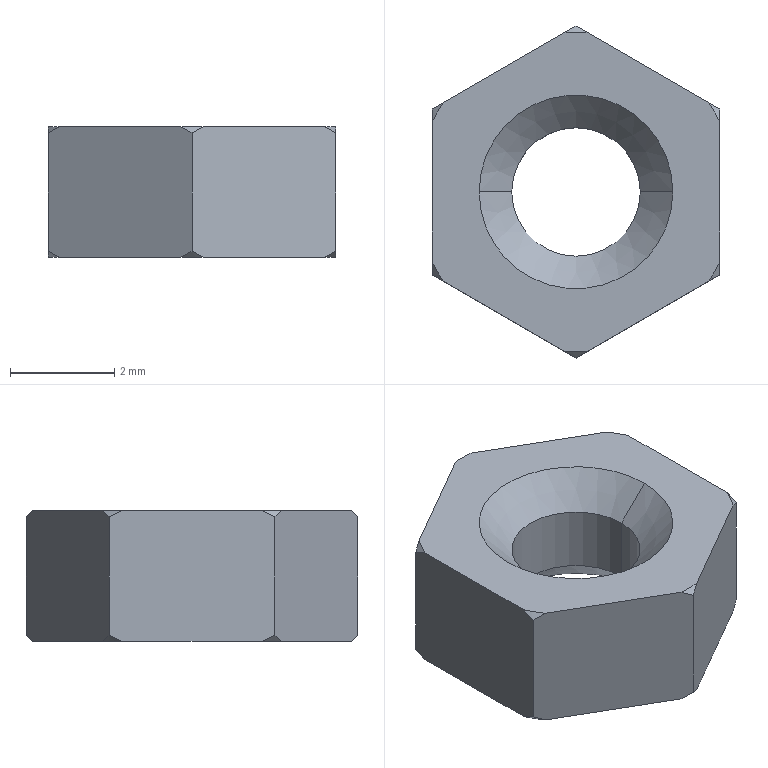Part | NX | features BREP 1 | 1 solid | 26 faces | box 5.5 x 6.351 x 2.5 mm | volume 50.092 mm3 | cone 16 | plane 8 | cylinder 2 | commonest cylinder face diameters 2.459 x2
STEP:
#1=CARTESIAN_POINT('',(-1.23,0.,-1.876));
#2=VERTEX_POINT('',#1);
#3=CARTESIAN_POINT('',(1.23,0.,-1.876));
#4=VERTEX_POINT('',#3);
#5=CARTESIAN_POINT('',(0.,0.,-1.876));
#6=DIRECTION('',(0.,0.,1.));
#7=DIRECTION('',(1.,0.,0.));
#8=AXIS2_PLACEMENT_3D('',#5,#6,#7);
#9=CIRCLE('',#8,1.23);
#10=EDGE_CURVE('',#2,#4,#9,.T.);
#11=ORIENTED_EDGE('',*,*,#10,.T.);
#12=CARTESIAN_POINT('',(1.854,0.,-2.5));
#13=VERTEX_POINT('',#12);
#14=CARTESIAN_POINT('',(1.23,0.,-1.876));
#15=DIRECTION('',(0.7071,0.,-0.7071));
#16=VECTOR('',#15,1000.);
#17=LINE('',#14,#16);
#18=EDGE_CURVE('',#13,#4,#17,.F.);
#19=ORIENTED_EDGE('',*,*,#18,.F.);
#20=CARTESIAN_POINT('',(-1.854,0.,-2.5));
#21=VERTEX_POINT('',#20);
#22=CARTESIAN_POINT('',(0.,0.,-2.5));
#23=DIRECTION('',(0.,0.,1.));
#24=DIRECTION('',(1.,0.,0.));
#25=AXIS2_PLACEMENT_3D('',#22,#23,#24);
#26=CIRCLE('',#25,1.854);
#27=EDGE_CURVE('',#21,#13,#26,.T.);
#28=ORIENTED_EDGE('',*,*,#27,.F.);
#29=CARTESIAN_POINT('',(-1.23,0.,-1.876));
#30=DIRECTION('',(-0.7071,0.,-0.7071));
#31=VECTOR('',#30,1000.);
#32=LINE('',#29,#31);
#33=EDGE_CURVE('',#21,#2,#32,.F.);
#34=ORIENTED_EDGE('',*,*,#33,.T.);
#35=EDGE_LOOP('',(#11,#19,#28,#34));
#36=FACE_BOUND('',#35,.T.);
#37=CARTESIAN_POINT('',(0.,0.,-1.876));
#38=DIRECTION('',(0.,0.,-1.));
#39=DIRECTION('',(1.,0.,0.));
#40=AXIS2_PLACEMENT_3D('',#37,#38,#39);
#41=CONICAL_SURFACE('',#40,1.23,0.7854);
#42=ADVANCED_FACE('',(#36),#41,.F.);
#43=ORIENTED_EDGE('',*,*,#10,.F.);
#44=CARTESIAN_POINT('',(-1.23,0.,-0.6241));
#45=VERTEX_POINT('',#44);
#46=CARTESIAN_POINT('',(-1.23,0.,-17.));
#47=DIRECTION('',(0.,0.,1.));
#48=VECTOR('',#47,1000.);
#49=LINE('',#46,#48);
#50=EDGE_CURVE('',#2,#45,#49,.T.);
#51=ORIENTED_EDGE('',*,*,#50,.T.);
#52=CARTESIAN_POINT('',(1.23,0.,-0.6241));
#53=VERTEX_POINT('',#52);
#54=CARTESIAN_POINT('',(0.,0.,-0.6241));
#55=DIRECTION('',(0.,0.,1.));
#56=DIRECTION('',(1.,0.,0.));
#57=AXIS2_PLACEMENT_3D('',#54,#55,#56);
#58=CIRCLE('',#57,1.23);
#59=EDGE_CURVE('',#45,#53,#58,.T.);
#60=ORIENTED_EDGE('',*,*,#59,.T.);
#61=CARTESIAN_POINT('',(1.23,0.,-17.));
#62=DIRECTION('',(0.,0.,1.));
#63=VECTOR('',#62,1000.);
#64=LINE('',#61,#63);
#65=EDGE_CURVE('',#4,#53,#64,.T.);
#66=ORIENTED_EDGE('',*,*,#65,.F.);
#67=EDGE_LOOP('',(#43,#51,#60,#66));
#68=FACE_BOUND('',#67,.T.);
#69=CARTESIAN_POINT('',(0.,0.,-17.));
#70=DIRECTION('',(0.,0.,1.));
#71=DIRECTION('',(-1.,0.,0.));
#72=AXIS2_PLACEMENT_3D('',#69,#70,#71);
#73=CYLINDRICAL_SURFACE('',#72,1.23);
#74=ADVANCED_FACE('',(#68),#73,.F.);
#75=ORIENTED_EDGE('',*,*,#59,.F.);
#76=CARTESIAN_POINT('',(-1.854,0.,0.));
#77=VERTEX_POINT('',#76);
#78=CARTESIAN_POINT('',(-1.854,0.,0.));
#79=DIRECTION('',(-0.7071,0.,0.7071));
#80=VECTOR('',#79,1000.);
#81=LINE('',#78,#80);
#82=EDGE_CURVE('',#45,#77,#81,.T.);
#83=ORIENTED_EDGE('',*,*,#82,.T.);
#84=CARTESIAN_POINT('',(1.854,0.,0.));
#85=VERTEX_POINT('',#84);
#86=CARTESIAN_POINT('',(0.,0.,0.));
#87=DIRECTION('',(0.,0.,1.));
#88=DIRECTION('',(1.,0.,0.));
#89=AXIS2_PLACEMENT_3D('',#86,#87,#88);
#90=CIRCLE('',#89,1.854);
#91=EDGE_CURVE('',#77,#85,#90,.T.);
#92=ORIENTED_EDGE('',*,*,#91,.T.);
#93=CARTESIAN_POINT('',(1.854,0.,0.));
#94=DIRECTION('',(0.7071,0.,0.7071));
#95=VECTOR('',#94,1000.);
#96=LINE('',#93,#95);
#97=EDGE_CURVE('',#53,#85,#96,.T.);
#98=ORIENTED_EDGE('',*,*,#97,.F.);
#99=EDGE_LOOP('',(#75,#83,#92,#98));
#100=FACE_BOUND('',#99,.T.);
#101=CARTESIAN_POINT('',(0.,0.,0.));
#102=DIRECTION('',(0.,0.,1.));
#103=DIRECTION('',(-1.,0.,0.));
#104=AXIS2_PLACEMENT_3D('',#101,#102,#103);
#105=CONICAL_SURFACE('',#104,1.854,0.7854);
#106=ADVANCED_FACE('',(#100),#105,.F.);
#107=CARTESIAN_POINT('',(-2.75,1.344,0.));
#108=VERTEX_POINT('',#107);
#109=CARTESIAN_POINT('',(-2.75,1.588,-0.1147));
#110=VERTEX_POINT('',#109);
#111=CARTESIAN_POINT('',(-2.75,1.344,0.));
#112=CARTESIAN_POINT('',(-2.75,1.426,-0.03612));
#113=CARTESIAN_POINT('',(-2.75,1.507,-0.07447));
#114=CARTESIAN_POINT('',(-2.75,1.588,-0.1147));
#115=B_SPLINE_CURVE_WITH_KNOTS('',3,(#111,#112,#113,#114),.UNSPECIFIED.,.F.,.F.,(4,4),(0.,1.),.PIECEWISE_BEZIER_KNOTS.);
#116=EDGE_CURVE('',#108,#110,#115,.T.);
#117=ORIENTED_EDGE('',*,*,#116,.F.);
#118=CARTESIAN_POINT('',(-2.539,1.71,0.));
#119=VERTEX_POINT('',#118);
#120=CARTESIAN_POINT('',(0.,0.,0.));
#121=DIRECTION('',(0.,0.,1.));
#122=DIRECTION('',(1.,0.,0.));
#123=AXIS2_PLACEMENT_3D('',#120,#121,#122);
#124=CIRCLE('',#123,3.061);
#125=EDGE_CURVE('',#119,#108,#124,.T.);
#126=ORIENTED_EDGE('',*,*,#125,.F.);
#127=CARTESIAN_POINT('',(-2.75,1.588,-0.1147));
#128=CARTESIAN_POINT('',(-2.68,1.628,-0.07445));
#129=CARTESIAN_POINT('',(-2.61,1.669,-0.03611));
#130=CARTESIAN_POINT('',(-2.539,1.71,0.));
#131=B_SPLINE_CURVE_WITH_KNOTS('',3,(#127,#128,#129,#130),.UNSPECIFIED.,.F.,.F.,(4,4),(0.,1.),.PIECEWISE_BEZIER_KNOTS.);
#132=EDGE_CURVE('',#110,#119,#131,.T.);
#133=ORIENTED_EDGE('',*,*,#132,.F.);
#134=EDGE_LOOP('',(#117,#126,#133));
#135=FACE_BOUND('',#134,.T.);
#136=CARTESIAN_POINT('',(0.,0.,-0.5893));
#137=DIRECTION('',(0.,0.,-1.));
#138=DIRECTION('',(1.,0.,0.));
#139=AXIS2_PLACEMENT_3D('',#136,#137,#138);
#140=CONICAL_SURFACE('',#139,3.65,0.7854);
#141=ADVANCED_FACE('',(#135),#140,.T.);
#142=CARTESIAN_POINT('',(-0.2113,3.053,0.));
#143=VERTEX_POINT('',#142);
#144=CARTESIAN_POINT('',(0.,3.175,-0.1147));
#145=VERTEX_POINT('',#144);
#146=CARTESIAN_POINT('',(-0.2113,3.053,0.));
#147=CARTESIAN_POINT('',(-0.1398,3.095,-0.03624));
#148=CARTESIAN_POINT('',(-0.06943,3.135,-0.07459));
#149=CARTESIAN_POINT('',(0.,3.175,-0.1147));
#150=B_SPLINE_CURVE_WITH_KNOTS('',3,(#146,#147,#148,#149),.UNSPECIFIED.,.F.,.F.,(4,4),(0.,1.),.PIECEWISE_BEZIER_KNOTS.);
#151=EDGE_CURVE('',#143,#145,#150,.T.);
#152=ORIENTED_EDGE('',*,*,#151,.F.);
#153=CARTESIAN_POINT('',(0.2113,3.053,0.));
#154=VERTEX_POINT('',#153);
#155=CARTESIAN_POINT('',(0.,0.,0.));
#156=DIRECTION('',(0.,0.,1.));
#157=DIRECTION('',(1.,0.,0.));
#158=AXIS2_PLACEMENT_3D('',#155,#156,#157);
#159=CIRCLE('',#158,3.061);
#160=EDGE_CURVE('',#154,#143,#159,.T.);
#161=ORIENTED_EDGE('',*,*,#160,.F.);
#162=CARTESIAN_POINT('',(0.,3.175,-0.1147));
#163=CARTESIAN_POINT('',(0.06968,3.135,-0.07445));
#164=CARTESIAN_POINT('',(0.1401,3.095,-0.03611));
#165=CARTESIAN_POINT('',(0.2113,3.053,0.));
#166=B_SPLINE_CURVE_WITH_KNOTS('',3,(#162,#163,#164,#165),.UNSPECIFIED.,.F.,.F.,(4,4),(0.,1.),.PIECEWISE_BEZIER_KNOTS.);
#167=EDGE_CURVE('',#145,#154,#166,.T.);
#168=ORIENTED_EDGE('',*,*,#167,.F.);
#169=EDGE_LOOP('',(#152,#161,#168));
#170=FACE_BOUND('',#169,.T.);
#171=CARTESIAN_POINT('',(0.,0.,-0.5893));
#172=DIRECTION('',(0.,0.,-1.));
#173=DIRECTION('',(1.,0.,0.));
#174=AXIS2_PLACEMENT_3D('',#171,#172,#173);
#175=CONICAL_SURFACE('',#174,3.65,0.7854);
#176=ADVANCED_FACE('',(#170),#175,.T.);
#177=CARTESIAN_POINT('',(2.539,1.71,0.));
#178=VERTEX_POINT('',#177);
#179=CARTESIAN_POINT('',(2.75,1.588,-0.1147));
#180=VERTEX_POINT('',#179);
#181=CARTESIAN_POINT('',(2.539,1.71,0.));
#182=CARTESIAN_POINT('',(2.61,1.668,-0.03624));
#183=CARTESIAN_POINT('',(2.681,1.628,-0.07459));
#184=CARTESIAN_POINT('',(2.75,1.588,-0.1147));
#185=B_SPLINE_CURVE_WITH_KNOTS('',3,(#181,#182,#183,#184),.UNSPECIFIED.,.F.,.F.,(4,4),(0.,1.),.PIECEWISE_BEZIER_KNOTS.);
#186=EDGE_CURVE('',#178,#180,#185,.T.);
#187=ORIENTED_EDGE('',*,*,#186,.F.);
#188=CARTESIAN_POINT('',(2.75,1.344,0.));
#189=VERTEX_POINT('',#188);
#190=CARTESIAN_POINT('',(0.,0.,0.));
#191=DIRECTION('',(0.,0.,1.));
#192=DIRECTION('',(1.,0.,0.));
#193=AXIS2_PLACEMENT_3D('',#190,#191,#192);
#194=CIRCLE('',#193,3.061);
#195=EDGE_CURVE('',#189,#178,#194,.T.);
#196=ORIENTED_EDGE('',*,*,#195,.F.);
#197=CARTESIAN_POINT('',(2.75,1.588,-0.1147));
#198=CARTESIAN_POINT('',(2.75,1.507,-0.07455));
#199=CARTESIAN_POINT('',(2.75,1.426,-0.03607));
#200=CARTESIAN_POINT('',(2.75,1.344,0.));
#201=B_SPLINE_CURVE_WITH_KNOTS('',3,(#197,#198,#199,#200),.UNSPECIFIED.,.F.,.F.,(4,4),(0.,1.),.PIECEWISE_BEZIER_KNOTS.);
#202=EDGE_CURVE('',#180,#189,#201,.T.);
#203=ORIENTED_EDGE('',*,*,#202,.F.);
#204=EDGE_LOOP('',(#187,#196,#203));
#205=FACE_BOUND('',#204,.T.);
#206=CARTESIAN_POINT('',(0.,0.,-0.5893));
#207=DIRECTION('',(0.,0.,-1.));
#208=DIRECTION('',(1.,0.,0.));
#209=AXIS2_PLACEMENT_3D('',#206,#207,#208);
#210=CONICAL_SURFACE('',#209,3.65,0.7854);
#211=ADVANCED_FACE('',(#205),#210,.T.);
#212=CARTESIAN_POINT('',(2.75,-1.344,0.));
#213=VERTEX_POINT('',#212);
#214=CARTESIAN_POINT('',(2.75,-1.588,-0.1147));
#215=VERTEX_POINT('',#214);
#216=CARTESIAN_POINT('',(2.75,-1.344,0.));
#217=CARTESIAN_POINT('',(2.75,-1.426,-0.03612));
#218=CARTESIAN_POINT('',(2.75,-1.507,-0.07447));
#219=CARTESIAN_POINT('',(2.75,-1.588,-0.1147));
#220=B_SPLINE_CURVE_WITH_KNOTS('',3,(#216,#217,#218,#219),.UNSPECIFIED.,.F.,.F.,(4,4),(0.,1.),.PIECEWISE_BEZIER_KNOTS.);
#221=EDGE_CURVE('',#213,#215,#220,.T.);
#222=ORIENTED_EDGE('',*,*,#221,.F.);
#223=CARTESIAN_POINT('',(2.539,-1.71,0.));
#224=VERTEX_POINT('',#223);
#225=CARTESIAN_POINT('',(0.,0.,0.));
#226=DIRECTION('',(0.,0.,1.));
#227=DIRECTION('',(1.,0.,0.));
#228=AXIS2_PLACEMENT_3D('',#225,#226,#227);
#229=CIRCLE('',#228,3.061);
#230=EDGE_CURVE('',#224,#213,#229,.T.);
#231=ORIENTED_EDGE('',*,*,#230,.F.);
#232=CARTESIAN_POINT('',(2.75,-1.588,-0.1147));
#233=CARTESIAN_POINT('',(2.68,-1.628,-0.07445));
#234=CARTESIAN_POINT('',(2.61,-1.669,-0.03611));
#235=CARTESIAN_POINT('',(2.539,-1.71,0.));
#236=B_SPLINE_CURVE_WITH_KNOTS('',3,(#232,#233,#234,#235),.UNSPECIFIED.,.F.,.F.,(4,4),(0.,1.),.PIECEWISE_BEZIER_KNOTS.);
#237=EDGE_CURVE('',#215,#224,#236,.T.);
#238=ORIENTED_EDGE('',*,*,#237,.F.);
#239=EDGE_LOOP('',(#222,#231,#238));
#240=FACE_BOUND('',#239,.T.);
#241=CARTESIAN_POINT('',(0.,0.,-0.5893));
#242=DIRECTION('',(0.,0.,-1.));
#243=DIRECTION('',(1.,0.,0.));
#244=AXIS2_PLACEMENT_3D('',#241,#242,#243);
#245=CONICAL_SURFACE('',#244,3.65,0.7854);
#246=ADVANCED_FACE('',(#240),#245,.T.);
#247=CARTESIAN_POINT('',(0.2113,-3.053,0.));
#248=VERTEX_POINT('',#247);
#249=CARTESIAN_POINT('',(0.,-3.175,-0.1147));
#250=VERTEX_POINT('',#249);
#251=CARTESIAN_POINT('',(0.2113,-3.053,0.));
#252=CARTESIAN_POINT('',(0.1398,-3.095,-0.03624));
#253=CARTESIAN_POINT('',(0.06943,-3.135,-0.07459));
#254=CARTESIAN_POINT('',(0.,-3.175,-0.1147));
#255=B_SPLINE_CURVE_WITH_KNOTS('',3,(#251,#252,#253,#254),.UNSPECIFIED.,.F.,.F.,(4,4),(0.,1.),.PIECEWISE_BEZIER_KNOTS.);
#256=EDGE_CURVE('',#248,#250,#255,.T.);
#257=ORIENTED_EDGE('',*,*,#256,.F.);
#258=CARTESIAN_POINT('',(-0.2113,-3.053,0.));
#259=VERTEX_POINT('',#258);
#260=CARTESIAN_POINT('',(0.,0.,0.));
#261=DIRECTION('',(0.,0.,1.));
#262=DIRECTION('',(1.,0.,0.));
#263=AXIS2_PLACEMENT_3D('',#260,#261,#262);
#264=CIRCLE('',#263,3.061);
#265=EDGE_CURVE('',#259,#248,#264,.T.);
#266=ORIENTED_EDGE('',*,*,#265,.F.);
#267=CARTESIAN_POINT('',(0.,-3.175,-0.1147));
#268=CARTESIAN_POINT('',(-0.06968,-3.135,-0.07445));
#269=CARTESIAN_POINT('',(-0.1401,-3.095,-0.03611));
#270=CARTESIAN_POINT('',(-0.2113,-3.053,0.));
#271=B_SPLINE_CURVE_WITH_KNOTS('',3,(#267,#268,#269,#270),.UNSPECIFIED.,.F.,.F.,(4,4),(0.,1.),.PIECEWISE_BEZIER_KNOTS.);
#272=EDGE_CURVE('',#250,#259,#271,.T.);
#273=ORIENTED_EDGE('',*,*,#272,.F.);
#274=EDGE_LOOP('',(#257,#266,#273));
#275=FACE_BOUND('',#274,.T.);
#276=CARTESIAN_POINT('',(0.,0.,-0.5893));
#277=DIRECTION('',(0.,0.,-1.));
#278=DIRECTION('',(1.,0.,0.));
#279=AXIS2_PLACEMENT_3D('',#276,#277,#278);
#280=CONICAL_SURFACE('',#279,3.65,0.7854);
#281=ADVANCED_FACE('',(#275),#280,.T.);
#282=CARTESIAN_POINT('',(-2.75,-1.588,-0.1147));
#283=VERTEX_POINT('',#282);
#284=CARTESIAN_POINT('',(-2.75,-1.344,0.));
#285=VERTEX_POINT('',#284);
#286=CARTESIAN_POINT('',(-2.75,-1.588,-0.1147));
#287=CARTESIAN_POINT('',(-2.75,-1.507,-0.07455));
#288=CARTESIAN_POINT('',(-2.75,-1.426,-0.03607));
#289=CARTESIAN_POINT('',(-2.75,-1.344,0.));
#290=B_SPLINE_CURVE_WITH_KNOTS('',3,(#286,#287,#288,#289),.UNSPECIFIED.,.F.,.F.,(4,4),(0.,1.),.PIECEWISE_BEZIER_KNOTS.);
#291=EDGE_CURVE('',#283,#285,#290,.T.);
#292=ORIENTED_EDGE('',*,*,#291,.F.);
#293=CARTESIAN_POINT('',(-2.539,-1.71,0.));
#294=VERTEX_POINT('',#293);
#295=CARTESIAN_POINT('',(-2.539,-1.71,0.));
#296=CARTESIAN_POINT('',(-2.61,-1.668,-0.03624));
#297=CARTESIAN_POINT('',(-2.681,-1.628,-0.07459));
#298=CARTESIAN_POINT('',(-2.75,-1.588,-0.1147));
#299=B_SPLINE_CURVE_WITH_KNOTS('',3,(#295,#296,#297,#298),.UNSPECIFIED.,.F.,.F.,(4,4),(0.,1.),.PIECEWISE_BEZIER_KNOTS.);
#300=EDGE_CURVE('',#294,#283,#299,.T.);
#301=ORIENTED_EDGE('',*,*,#300,.F.);
#302=CARTESIAN_POINT('',(0.,0.,0.));
#303=DIRECTION('',(0.,0.,1.));
#304=DIRECTION('',(1.,0.,0.));
#305=AXIS2_PLACEMENT_3D('',#302,#303,#304);
#306=CIRCLE('',#305,3.061);
#307=EDGE_CURVE('',#285,#294,#306,.T.);
#308=ORIENTED_EDGE('',*,*,#307,.F.);
#309=EDGE_LOOP('',(#292,#301,#308));
#310=FACE_BOUND('',#309,.T.);
#311=CARTESIAN_POINT('',(0.,0.,-0.5893));
#312=DIRECTION('',(0.,0.,-1.));
#313=DIRECTION('',(1.,0.,0.));
#314=AXIS2_PLACEMENT_3D('',#311,#312,#313);
#315=CONICAL_SURFACE('',#314,3.65,0.7854);
#316=ADVANCED_FACE('',(#310),#315,.T.);
#317=CARTESIAN_POINT('',(0.,0.,0.));
#318=DIRECTION('',(0.,0.,1.));
#319=DIRECTION('',(1.,0.,0.));
#320=AXIS2_PLACEMENT_3D('',#317,#318,#319);
#321=CIRCLE('',#320,1.854);
#322=EDGE_CURVE('',#85,#77,#321,.T.);
#323=ORIENTED_EDGE('',*,*,#322,.F.);
#324=ORIENTED_EDGE('',*,*,#91,.F.);
#325=EDGE_LOOP('',(#323,#324));
#326=FACE_BOUND('',#325,.T.);
#327=CARTESIAN_POINT('',(-2.75,1.588,0.));
#328=DIRECTION('',(0.,-1.,0.));
#329=VECTOR('',#328,1000.);
#330=LINE('',#327,#329);
#331=EDGE_CURVE('',#108,#285,#330,.T.);
#332=ORIENTED_EDGE('',*,*,#331,.T.);
#333=ORIENTED_EDGE('',*,*,#307,.T.);
#334=CARTESIAN_POINT('',(-2.75,-1.588,0.));
#335=DIRECTION('',(0.866,-0.5,0.));
#336=VECTOR('',#335,1000.);
#337=LINE('',#334,#336);
#338=EDGE_CURVE('',#294,#259,#337,.T.);
#339=ORIENTED_EDGE('',*,*,#338,.T.);
#340=ORIENTED_EDGE('',*,*,#265,.T.);
#341=CARTESIAN_POINT('',(0.,-3.175,0.));
#342=DIRECTION('',(0.866,0.5,0.));
#343=VECTOR('',#342,1000.);
#344=LINE('',#341,#343);
#345=EDGE_CURVE('',#248,#224,#344,.T.);
#346=ORIENTED_EDGE('',*,*,#345,.T.);
#347=ORIENTED_EDGE('',*,*,#230,.T.);
#348=CARTESIAN_POINT('',(2.75,-1.588,0.));
#349=DIRECTION('',(0.,1.,0.));
#350=VECTOR('',#349,1000.);
#351=LINE('',#348,#350);
#352=EDGE_CURVE('',#213,#189,#351,.T.);
#353=ORIENTED_EDGE('',*,*,#352,.T.);
#354=ORIENTED_EDGE('',*,*,#195,.T.);
#355=CARTESIAN_POINT('',(2.75,1.588,0.));
#356=DIRECTION('',(-0.866,0.5,0.));
#357=VECTOR('',#356,1000.);
#358=LINE('',#355,#357);
#359=EDGE_CURVE('',#178,#154,#358,.T.);
#360=ORIENTED_EDGE('',*,*,#359,.T.);
#361=ORIENTED_EDGE('',*,*,#160,.T.);
#362=CARTESIAN_POINT('',(0.,3.175,0.));
#363=DIRECTION('',(-0.866,-0.5,0.));
#364=VECTOR('',#363,1000.);
#365=LINE('',#362,#364);
#366=EDGE_CURVE('',#143,#119,#365,.T.);
#367=ORIENTED_EDGE('',*,*,#366,.T.);
#368=ORIENTED_EDGE('',*,*,#125,.T.);
#369=EDGE_LOOP('',(#332,#333,#339,#340,#346,#347,#353,#354,#360,#361,#367,#368));
#370=FACE_BOUND('',#369,.T.);
#371=CARTESIAN_POINT('',(0.,3.061,0.));
#372=DIRECTION('',(0.,0.,-1.));
#373=DIRECTION('',(1.,0.,0.));
#374=AXIS2_PLACEMENT_3D('',#371,#372,#373);
#375=PLANE('',#374);
#376=ADVANCED_FACE('',(#326,#370),#375,.F.);
#377=ORIENTED_EDGE('',*,*,#27,.T.);
#378=CARTESIAN_POINT('',(0.,0.,-2.5));
#379=DIRECTION('',(0.,0.,1.));
#380=DIRECTION('',(1.,0.,0.));
#381=AXIS2_PLACEMENT_3D('',#378,#379,#380);
#382=CIRCLE('',#381,1.854);
#383=EDGE_CURVE('',#13,#21,#382,.T.);
#384=ORIENTED_EDGE('',*,*,#383,.T.);
#385=EDGE_LOOP('',(#377,#384));
#386=FACE_BOUND('',#385,.T.);
#387=CARTESIAN_POINT('',(-2.75,1.344,-2.5));
#388=VERTEX_POINT('',#387);
#389=CARTESIAN_POINT('',(-2.75,-1.344,-2.5));
#390=VERTEX_POINT('',#389);
#391=CARTESIAN_POINT('',(-2.75,1.854,-2.5));
#392=DIRECTION('',(0.,-1.,0.));
#393=VECTOR('',#392,1000.);
#394=LINE('',#391,#393);
#395=EDGE_CURVE('',#388,#390,#394,.T.);
#396=ORIENTED_EDGE('',*,*,#395,.F.);
#397=CARTESIAN_POINT('',(-2.539,1.71,-2.5));
#398=VERTEX_POINT('',#397);
#399=CARTESIAN_POINT('',(0.,0.,-2.5));
#400=DIRECTION('',(0.,0.,1.));
#401=DIRECTION('',(1.,0.,0.));
#402=AXIS2_PLACEMENT_3D('',#399,#400,#401);
#403=CIRCLE('',#402,3.061);
#404=EDGE_CURVE('',#398,#388,#403,.T.);
#405=ORIENTED_EDGE('',*,*,#404,.F.);
#406=CARTESIAN_POINT('',(-0.2113,3.053,-2.5));
#407=VERTEX_POINT('',#406);
#408=CARTESIAN_POINT('',(-0.5724,2.845,-2.5));
#409=DIRECTION('',(-0.866,-0.5,0.));
#410=VECTOR('',#409,1000.);
#411=LINE('',#408,#410);
#412=EDGE_CURVE('',#407,#398,#411,.T.);
#413=ORIENTED_EDGE('',*,*,#412,.F.);
#414=CARTESIAN_POINT('',(0.2113,3.053,-2.5));
#415=VERTEX_POINT('',#414);
#416=CARTESIAN_POINT('',(0.,0.,-2.5));
#417=DIRECTION('',(0.,0.,1.));
#418=DIRECTION('',(1.,0.,0.));
#419=AXIS2_PLACEMENT_3D('',#416,#417,#418);
#420=CIRCLE('',#419,3.061);
#421=EDGE_CURVE('',#415,#407,#420,.T.);
#422=ORIENTED_EDGE('',*,*,#421,.F.);
#423=CARTESIAN_POINT('',(2.539,1.71,-2.5));
#424=VERTEX_POINT('',#423);
#425=CARTESIAN_POINT('',(0.5724,2.845,-2.5));
#426=DIRECTION('',(-0.866,0.5,0.));
#427=VECTOR('',#426,1000.);
#428=LINE('',#425,#427);
#429=EDGE_CURVE('',#424,#415,#428,.T.);
#430=ORIENTED_EDGE('',*,*,#429,.F.);
#431=CARTESIAN_POINT('',(2.75,1.344,-2.5));
#432=VERTEX_POINT('',#431);
#433=CARTESIAN_POINT('',(0.,0.,-2.5));
#434=DIRECTION('',(0.,0.,1.));
#435=DIRECTION('',(1.,0.,0.));
#436=AXIS2_PLACEMENT_3D('',#433,#434,#435);
#437=CIRCLE('',#436,3.061);
#438=EDGE_CURVE('',#432,#424,#437,.T.);
#439=ORIENTED_EDGE('',*,*,#438,.F.);
#440=CARTESIAN_POINT('',(2.75,-1.344,-2.5));
#441=VERTEX_POINT('',#440);
#442=CARTESIAN_POINT('',(2.75,1.854,-2.5));
#443=DIRECTION('',(0.,1.,0.));
#444=VECTOR('',#443,1000.);
#445=LINE('',#442,#444);
#446=EDGE_CURVE('',#441,#432,#445,.T.);
#447=ORIENTED_EDGE('',*,*,#446,.F.);
#448=CARTESIAN_POINT('',(2.539,-1.71,-2.5));
#449=VERTEX_POINT('',#448);
#450=CARTESIAN_POINT('',(0.,0.,-2.5));
#451=DIRECTION('',(0.,0.,1.));
#452=DIRECTION('',(1.,0.,0.));
#453=AXIS2_PLACEMENT_3D('',#450,#451,#452);
#454=CIRCLE('',#453,3.061);
#455=EDGE_CURVE('',#449,#441,#454,.T.);
#456=ORIENTED_EDGE('',*,*,#455,.F.);
#457=CARTESIAN_POINT('',(0.2113,-3.053,-2.5));
#458=VERTEX_POINT('',#457);
#459=CARTESIAN_POINT('',(2.178,-1.918,-2.5));
#460=DIRECTION('',(0.866,0.5,0.));
#461=VECTOR('',#460,1000.);
#462=LINE('',#459,#461);
#463=EDGE_CURVE('',#458,#449,#462,.T.);
#464=ORIENTED_EDGE('',*,*,#463,.F.);
#465=CARTESIAN_POINT('',(-0.2113,-3.053,-2.5));
#466=VERTEX_POINT('',#465);
#467=CARTESIAN_POINT('',(0.,0.,-2.5));
#468=DIRECTION('',(0.,0.,1.));
#469=DIRECTION('',(1.,0.,0.));
#470=AXIS2_PLACEMENT_3D('',#467,#468,#469);
#471=CIRCLE('',#470,3.061);
#472=EDGE_CURVE('',#466,#458,#471,.T.);
#473=ORIENTED_EDGE('',*,*,#472,.F.);
#474=CARTESIAN_POINT('',(-2.539,-1.71,-2.5));
#475=VERTEX_POINT('',#474);
#476=CARTESIAN_POINT('',(-2.178,-1.918,-2.5));
#477=DIRECTION('',(0.866,-0.5,0.));
#478=VECTOR('',#477,1000.);
#479=LINE('',#476,#478);
#480=EDGE_CURVE('',#475,#466,#479,.T.);
#481=ORIENTED_EDGE('',*,*,#480,.F.);
#482=CARTESIAN_POINT('',(0.,0.,-2.5));
#483=DIRECTION('',(0.,0.,1.));
#484=DIRECTION('',(1.,0.,0.));
#485=AXIS2_PLACEMENT_3D('',#482,#483,#484);
#486=CIRCLE('',#485,3.061);
#487=EDGE_CURVE('',#390,#475,#486,.T.);
#488=ORIENTED_EDGE('',*,*,#487,.F.);
#489=EDGE_LOOP('',(#396,#405,#413,#422,#430,#439,#447,#456,#464,#473,#481,#488));
#490=FACE_BOUND('',#489,.T.);
#491=CARTESIAN_POINT('',(0.,1.854,-2.5));
#492=DIRECTION('',(0.,0.,1.));
#493=DIRECTION('',(-1.,0.,0.));
#494=AXIS2_PLACEMENT_3D('',#491,#492,#493);
#495=PLANE('',#494);
#496=ADVANCED_FACE('',(#386,#490),#495,.F.);
#497=CARTESIAN_POINT('',(-2.75,1.588,-2.385));
#498=VERTEX_POINT('',#497);
#499=CARTESIAN_POINT('',(-2.75,1.588,-2.385));
#500=CARTESIAN_POINT('',(-2.75,1.507,-2.425));
#501=CARTESIAN_POINT('',(-2.75,1.426,-2.464));
#502=CARTESIAN_POINT('',(-2.75,1.344,-2.5));
#503=B_SPLINE_CURVE_WITH_KNOTS('',3,(#499,#500,#501,#502),.UNSPECIFIED.,.F.,.F.,(4,4),(0.,1.),.PIECEWISE_BEZIER_KNOTS.);
#504=EDGE_CURVE('',#498,#388,#503,.T.);
#505=ORIENTED_EDGE('',*,*,#504,.F.);
#506=CARTESIAN_POINT('',(-2.539,1.71,-2.5));
#507=CARTESIAN_POINT('',(-2.61,1.668,-2.464));
#508=CARTESIAN_POINT('',(-2.681,1.628,-2.425));
#509=CARTESIAN_POINT('',(-2.75,1.588,-2.385));
#510=B_SPLINE_CURVE_WITH_KNOTS('',3,(#506,#507,#508,#509),.UNSPECIFIED.,.F.,.F.,(4,4),(0.,1.),.PIECEWISE_BEZIER_KNOTS.);
#511=EDGE_CURVE('',#398,#498,#510,.T.);
#512=ORIENTED_EDGE('',*,*,#511,.F.);
#513=ORIENTED_EDGE('',*,*,#404,.T.);
#514=EDGE_LOOP('',(#505,#512,#513));
#515=FACE_BOUND('',#514,.T.);
#516=CARTESIAN_POINT('',(0.,0.,-2.5));
#517=DIRECTION('',(0.,0.,1.));
#518=DIRECTION('',(-1.,0.,0.));
#519=AXIS2_PLACEMENT_3D('',#516,#517,#518);
#520=CONICAL_SURFACE('',#519,3.061,0.7854);
#521=ADVANCED_FACE('',(#515),#520,.T.);
#522=CARTESIAN_POINT('',(0.,3.175,-2.385));
#523=VERTEX_POINT('',#522);
#524=CARTESIAN_POINT('',(0.,3.175,-2.385));
#525=CARTESIAN_POINT('',(-0.06968,3.135,-2.426));
#526=CARTESIAN_POINT('',(-0.1401,3.095,-2.464));
#527=CARTESIAN_POINT('',(-0.2113,3.053,-2.5));
#528=B_SPLINE_CURVE_WITH_KNOTS('',3,(#524,#525,#526,#527),.UNSPECIFIED.,.F.,.F.,(4,4),(0.,1.),.PIECEWISE_BEZIER_KNOTS.);
#529=EDGE_CURVE('',#523,#407,#528,.T.);
#530=ORIENTED_EDGE('',*,*,#529,.F.);
#531=CARTESIAN_POINT('',(0.2113,3.053,-2.5));
#532=CARTESIAN_POINT('',(0.1398,3.095,-2.464));
#533=CARTESIAN_POINT('',(0.06943,3.135,-2.425));
#534=CARTESIAN_POINT('',(0.,3.175,-2.385));
#535=B_SPLINE_CURVE_WITH_KNOTS('',3,(#531,#532,#533,#534),.UNSPECIFIED.,.F.,.F.,(4,4),(0.,1.),.PIECEWISE_BEZIER_KNOTS.);
#536=EDGE_CURVE('',#415,#523,#535,.T.);
#537=ORIENTED_EDGE('',*,*,#536,.F.);
#538=ORIENTED_EDGE('',*,*,#421,.T.);
#539=EDGE_LOOP('',(#530,#537,#538));
#540=FACE_BOUND('',#539,.T.);
#541=CARTESIAN_POINT('',(0.,0.,-2.5));
#542=DIRECTION('',(0.,0.,1.));
#543=DIRECTION('',(-1.,0.,0.));
#544=AXIS2_PLACEMENT_3D('',#541,#542,#543);
#545=CONICAL_SURFACE('',#544,3.061,0.7854);
#546=ADVANCED_FACE('',(#540),#545,.T.);
#547=CARTESIAN_POINT('',(2.75,1.588,-2.385));
#548=VERTEX_POINT('',#547);
#549=CARTESIAN_POINT('',(2.75,1.588,-2.385));
#550=CARTESIAN_POINT('',(2.68,1.628,-2.426));
#551=CARTESIAN_POINT('',(2.61,1.669,-2.464));
#552=CARTESIAN_POINT('',(2.539,1.71,-2.5));
#553=B_SPLINE_CURVE_WITH_KNOTS('',3,(#549,#550,#551,#552),.UNSPECIFIED.,.F.,.F.,(4,4),(0.,1.),.PIECEWISE_BEZIER_KNOTS.);
#554=EDGE_CURVE('',#548,#424,#553,.T.);
#555=ORIENTED_EDGE('',*,*,#554,.F.);
#556=CARTESIAN_POINT('',(2.75,1.344,-2.5));
#557=CARTESIAN_POINT('',(2.75,1.426,-2.464));
#558=CARTESIAN_POINT('',(2.75,1.507,-2.426));
#559=CARTESIAN_POINT('',(2.75,1.588,-2.385));
#560=B_SPLINE_CURVE_WITH_KNOTS('',3,(#556,#557,#558,#559),.UNSPECIFIED.,.F.,.F.,(4,4),(0.,1.),.PIECEWISE_BEZIER_KNOTS.);
#561=EDGE_CURVE('',#432,#548,#560,.T.);
#562=ORIENTED_EDGE('',*,*,#561,.F.);
#563=ORIENTED_EDGE('',*,*,#438,.T.);
#564=EDGE_LOOP('',(#555,#562,#563));
#565=FACE_BOUND('',#564,.T.);
#566=CARTESIAN_POINT('',(0.,0.,-2.5));
#567=DIRECTION('',(0.,0.,1.));
#568=DIRECTION('',(-1.,0.,0.));
#569=AXIS2_PLACEMENT_3D('',#566,#567,#568);
#570=CONICAL_SURFACE('',#569,3.061,0.7854);
#571=ADVANCED_FACE('',(#565),#570,.T.);
#572=CARTESIAN_POINT('',(2.75,-1.588,-2.385));
#573=VERTEX_POINT('',#572);
#574=CARTESIAN_POINT('',(2.75,-1.588,-2.385));
#575=CARTESIAN_POINT('',(2.75,-1.507,-2.425));
#576=CARTESIAN_POINT('',(2.75,-1.426,-2.464));
#577=CARTESIAN_POINT('',(2.75,-1.344,-2.5));
#578=B_SPLINE_CURVE_WITH_KNOTS('',3,(#574,#575,#576,#577),.UNSPECIFIED.,.F.,.F.,(4,4),(0.,1.),.PIECEWISE_BEZIER_KNOTS.);
#579=EDGE_CURVE('',#573,#441,#578,.T.);
#580=ORIENTED_EDGE('',*,*,#579,.F.);
#581=CARTESIAN_POINT('',(2.539,-1.71,-2.5));
#582=CARTESIAN_POINT('',(2.61,-1.668,-2.464));
#583=CARTESIAN_POINT('',(2.681,-1.628,-2.425));
#584=CARTESIAN_POINT('',(2.75,-1.588,-2.385));
#585=B_SPLINE_CURVE_WITH_KNOTS('',3,(#581,#582,#583,#584),.UNSPECIFIED.,.F.,.F.,(4,4),(0.,1.),.PIECEWISE_BEZIER_KNOTS.);
#586=EDGE_CURVE('',#449,#573,#585,.T.);
#587=ORIENTED_EDGE('',*,*,#586,.F.);
#588=ORIENTED_EDGE('',*,*,#455,.T.);
#589=EDGE_LOOP('',(#580,#587,#588));
#590=FACE_BOUND('',#589,.T.);
#591=CARTESIAN_POINT('',(0.,0.,-2.5));
#592=DIRECTION('',(0.,0.,1.));
#593=DIRECTION('',(-1.,0.,0.));
#594=AXIS2_PLACEMENT_3D('',#591,#592,#593);
#595=CONICAL_SURFACE('',#594,3.061,0.7854);
#596=ADVANCED_FACE('',(#590),#595,.T.);
#597=CARTESIAN_POINT('',(-2.75,-1.588,-2.385));
#598=VERTEX_POINT('',#597);
#599=CARTESIAN_POINT('',(-2.75,-1.344,-2.5));
#600=CARTESIAN_POINT('',(-2.75,-1.426,-2.464));
#601=CARTESIAN_POINT('',(-2.75,-1.507,-2.426));
#602=CARTESIAN_POINT('',(-2.75,-1.588,-2.385));
#603=B_SPLINE_CURVE_WITH_KNOTS('',3,(#599,#600,#601,#602),.UNSPECIFIED.,.F.,.F.,(4,4),(0.,1.),.PIECEWISE_BEZIER_KNOTS.);
#604=EDGE_CURVE('',#390,#598,#603,.T.);
#605=ORIENTED_EDGE('',*,*,#604,.F.);
#606=ORIENTED_EDGE('',*,*,#487,.T.);
#607=CARTESIAN_POINT('',(-2.75,-1.588,-2.385));
#608=CARTESIAN_POINT('',(-2.68,-1.628,-2.426));
#609=CARTESIAN_POINT('',(-2.61,-1.669,-2.464));
#610=CARTESIAN_POINT('',(-2.539,-1.71,-2.5));
#611=B_SPLINE_CURVE_WITH_KNOTS('',3,(#607,#608,#609,#610),.UNSPECIFIED.,.F.,.F.,(4,4),(0.,1.),.PIECEWISE_BEZIER_KNOTS.);
#612=EDGE_CURVE('',#598,#475,#611,.T.);
#613=ORIENTED_EDGE('',*,*,#612,.F.);
#614=EDGE_LOOP('',(#605,#606,#613));
#615=FACE_BOUND('',#614,.T.);
#616=CARTESIAN_POINT('',(0.,0.,-2.5));
#617=DIRECTION('',(0.,0.,1.));
#618=DIRECTION('',(-1.,0.,0.));
#619=AXIS2_PLACEMENT_3D('',#616,#617,#618);
#620=CONICAL_SURFACE('',#619,3.061,0.7854);
#621=ADVANCED_FACE('',(#615),#620,.T.);
#622=CARTESIAN_POINT('',(0.,-3.175,-2.385));
#623=VERTEX_POINT('',#622);
#624=CARTESIAN_POINT('',(0.,-3.175,-2.385));
#625=CARTESIAN_POINT('',(0.06968,-3.135,-2.426));
#626=CARTESIAN_POINT('',(0.1401,-3.095,-2.464));
#627=CARTESIAN_POINT('',(0.2113,-3.053,-2.5));
#628=B_SPLINE_CURVE_WITH_KNOTS('',3,(#624,#625,#626,#627),.UNSPECIFIED.,.F.,.F.,(4,4),(0.,1.),.PIECEWISE_BEZIER_KNOTS.);
#629=EDGE_CURVE('',#623,#458,#628,.T.);
#630=ORIENTED_EDGE('',*,*,#629,.F.);
#631=CARTESIAN_POINT('',(-0.2113,-3.053,-2.5));
#632=CARTESIAN_POINT('',(-0.1398,-3.095,-2.464));
#633=CARTESIAN_POINT('',(-0.06943,-3.135,-2.425));
#634=CARTESIAN_POINT('',(0.,-3.175,-2.385));
#635=B_SPLINE_CURVE_WITH_KNOTS('',3,(#631,#632,#633,#634),.UNSPECIFIED.,.F.,.F.,(4,4),(0.,1.),.PIECEWISE_BEZIER_KNOTS.);
#636=EDGE_CURVE('',#466,#623,#635,.T.);
#637=ORIENTED_EDGE('',*,*,#636,.F.);
#638=ORIENTED_EDGE('',*,*,#472,.T.);
#639=EDGE_LOOP('',(#630,#637,#638));
#640=FACE_BOUND('',#639,.T.);
#641=CARTESIAN_POINT('',(0.,0.,-2.5));
#642=DIRECTION('',(0.,0.,1.));
#643=DIRECTION('',(-1.,0.,0.));
#644=AXIS2_PLACEMENT_3D('',#641,#642,#643);
#645=CONICAL_SURFACE('',#644,3.061,0.7854);
#646=ADVANCED_FACE('',(#640),#645,.T.);
#647=ORIENTED_EDGE('',*,*,#82,.F.);
#648=CARTESIAN_POINT('',(0.,0.,-0.6241));
#649=DIRECTION('',(0.,0.,1.));
#650=DIRECTION('',(1.,0.,0.));
#651=AXIS2_PLACEMENT_3D('',#648,#649,#650);
#652=CIRCLE('',#651,1.23);
#653=EDGE_CURVE('',#53,#45,#652,.T.);
#654=ORIENTED_EDGE('',*,*,#653,.F.);
#655=ORIENTED_EDGE('',*,*,#97,.T.);
#656=ORIENTED_EDGE('',*,*,#322,.T.);
#657=EDGE_LOOP('',(#647,#654,#655,#656));
#658=FACE_BOUND('',#657,.T.);
#659=CARTESIAN_POINT('',(0.,0.,0.));
#660=DIRECTION('',(0.,0.,1.));
#661=DIRECTION('',(-1.,0.,0.));
#662=AXIS2_PLACEMENT_3D('',#659,#660,#661);
#663=CONICAL_SURFACE('',#662,1.854,0.7854);
#664=ADVANCED_FACE('',(#658),#663,.F.);
#665=ORIENTED_EDGE('',*,*,#50,.F.);
#666=CARTESIAN_POINT('',(0.,0.,-1.876));
#667=DIRECTION('',(0.,0.,1.));
#668=DIRECTION('',(1.,0.,0.));
#669=AXIS2_PLACEMENT_3D('',#666,#667,#668);
#670=CIRCLE('',#669,1.23);
#671=EDGE_CURVE('',#4,#2,#670,.T.);
#672=ORIENTED_EDGE('',*,*,#671,.F.);
#673=ORIENTED_EDGE('',*,*,#65,.T.);
#674=ORIENTED_EDGE('',*,*,#653,.T.);
#675=EDGE_LOOP('',(#665,#672,#673,#674));
#676=FACE_BOUND('',#675,.T.);
#677=CARTESIAN_POINT('',(0.,0.,-17.));
#678=DIRECTION('',(0.,0.,1.));
#679=DIRECTION('',(-1.,0.,0.));
#680=AXIS2_PLACEMENT_3D('',#677,#678,#679);
#681=CYLINDRICAL_SURFACE('',#680,1.23);
#682=ADVANCED_FACE('',(#676),#681,.F.);
#683=ORIENTED_EDGE('',*,*,#18,.T.);
#684=ORIENTED_EDGE('',*,*,#671,.T.);
#685=ORIENTED_EDGE('',*,*,#33,.F.);
#686=ORIENTED_EDGE('',*,*,#383,.F.);
#687=EDGE_LOOP('',(#683,#684,#685,#686));
#688=FACE_BOUND('',#687,.T.);
#689=CARTESIAN_POINT('',(0.,0.,-1.876));
#690=DIRECTION('',(0.,0.,-1.));
#691=DIRECTION('',(1.,0.,0.));
#692=AXIS2_PLACEMENT_3D('',#689,#690,#691);
#693=CONICAL_SURFACE('',#692,1.23,0.7854);
#694=ADVANCED_FACE('',(#688),#693,.F.);
#695=ORIENTED_EDGE('',*,*,#291,.T.);
#696=ORIENTED_EDGE('',*,*,#331,.F.);
#697=ORIENTED_EDGE('',*,*,#116,.T.);
#698=CARTESIAN_POINT('',(-2.75,1.588,-4.));
#699=DIRECTION('',(0.,0.,1.));
#700=VECTOR('',#699,1000.);
#701=LINE('',#698,#700);
#702=EDGE_CURVE('',#498,#110,#701,.T.);
#703=ORIENTED_EDGE('',*,*,#702,.F.);
#704=ORIENTED_EDGE('',*,*,#504,.T.);
#705=ORIENTED_EDGE('',*,*,#395,.T.);
#706=ORIENTED_EDGE('',*,*,#604,.T.);
#707=CARTESIAN_POINT('',(-2.75,-1.588,-4.));
#708=DIRECTION('',(0.,0.,1.));
#709=VECTOR('',#708,1000.);
#710=LINE('',#707,#709);
#711=EDGE_CURVE('',#598,#283,#710,.T.);
#712=ORIENTED_EDGE('',*,*,#711,.T.);
#713=EDGE_LOOP('',(#695,#696,#697,#703,#704,#705,#706,#712));
#714=FACE_BOUND('',#713,.T.);
#715=CARTESIAN_POINT('',(-2.75,1.588,-4.));
#716=DIRECTION('',(-1.,0.,0.));
#717=DIRECTION('',(0.,0.,-1.));
#718=AXIS2_PLACEMENT_3D('',#715,#716,#717);
#719=PLANE('',#718);
#720=ADVANCED_FACE('',(#714),#719,.T.);
#721=ORIENTED_EDGE('',*,*,#132,.T.);
#722=ORIENTED_EDGE('',*,*,#366,.F.);
#723=ORIENTED_EDGE('',*,*,#151,.T.);
#724=CARTESIAN_POINT('',(0.,3.175,-4.));
#725=DIRECTION('',(0.,0.,1.));
#726=VECTOR('',#725,1000.);
#727=LINE('',#724,#726);
#728=EDGE_CURVE('',#523,#145,#727,.T.);
#729=ORIENTED_EDGE('',*,*,#728,.F.);
#730=ORIENTED_EDGE('',*,*,#529,.T.);
#731=ORIENTED_EDGE('',*,*,#412,.T.);
#732=ORIENTED_EDGE('',*,*,#511,.T.);
#733=ORIENTED_EDGE('',*,*,#702,.T.);
#734=EDGE_LOOP('',(#721,#722,#723,#729,#730,#731,#732,#733));
#735=FACE_BOUND('',#734,.T.);
#736=CARTESIAN_POINT('',(0.,3.175,-4.));
#737=DIRECTION('',(-0.5,0.866,0.));
#738=DIRECTION('',(0.866,0.5,0.));
#739=AXIS2_PLACEMENT_3D('',#736,#737,#738);
#740=PLANE('',#739);
#741=ADVANCED_FACE('',(#735),#740,.T.);
#742=ORIENTED_EDGE('',*,*,#167,.T.);
#743=ORIENTED_EDGE('',*,*,#359,.F.);
#744=ORIENTED_EDGE('',*,*,#186,.T.);
#745=CARTESIAN_POINT('',(2.75,1.588,-4.));
#746=DIRECTION('',(0.,0.,1.));
#747=VECTOR('',#746,1000.);
#748=LINE('',#745,#747);
#749=EDGE_CURVE('',#548,#180,#748,.T.);
#750=ORIENTED_EDGE('',*,*,#749,.F.);
#751=ORIENTED_EDGE('',*,*,#554,.T.);
#752=ORIENTED_EDGE('',*,*,#429,.T.);
#753=ORIENTED_EDGE('',*,*,#536,.T.);
#754=ORIENTED_EDGE('',*,*,#728,.T.);
#755=EDGE_LOOP('',(#742,#743,#744,#750,#751,#752,#753,#754));
#756=FACE_BOUND('',#755,.T.);
#757=CARTESIAN_POINT('',(2.75,1.588,-4.));
#758=DIRECTION('',(0.5,0.866,0.));
#759=DIRECTION('',(0.866,-0.5,0.));
#760=AXIS2_PLACEMENT_3D('',#757,#758,#759);
#761=PLANE('',#760);
#762=ADVANCED_FACE('',(#756),#761,.T.);
#763=ORIENTED_EDGE('',*,*,#202,.T.);
#764=ORIENTED_EDGE('',*,*,#352,.F.);
#765=ORIENTED_EDGE('',*,*,#221,.T.);
#766=CARTESIAN_POINT('',(2.75,-1.588,-4.));
#767=DIRECTION('',(0.,0.,1.));
#768=VECTOR('',#767,1000.);
#769=LINE('',#766,#768);
#770=EDGE_CURVE('',#573,#215,#769,.T.);
#771=ORIENTED_EDGE('',*,*,#770,.F.);
#772=ORIENTED_EDGE('',*,*,#579,.T.);
#773=ORIENTED_EDGE('',*,*,#446,.T.);
#774=ORIENTED_EDGE('',*,*,#561,.T.);
#775=ORIENTED_EDGE('',*,*,#749,.T.);
#776=EDGE_LOOP('',(#763,#764,#765,#771,#772,#773,#774,#775));
#777=FACE_BOUND('',#776,.T.);
#778=CARTESIAN_POINT('',(2.75,-1.588,-4.));
#779=DIRECTION('',(1.,0.,0.));
#780=DIRECTION('',(0.,0.,1.));
#781=AXIS2_PLACEMENT_3D('',#778,#779,#780);
#782=PLANE('',#781);
#783=ADVANCED_FACE('',(#777),#782,.T.);
#784=ORIENTED_EDGE('',*,*,#237,.T.);
#785=ORIENTED_EDGE('',*,*,#345,.F.);
#786=ORIENTED_EDGE('',*,*,#256,.T.);
#787=CARTESIAN_POINT('',(0.,-3.175,-4.));
#788=DIRECTION('',(0.,0.,1.));
#789=VECTOR('',#788,1000.);
#790=LINE('',#787,#789);
#791=EDGE_CURVE('',#623,#250,#790,.T.);
#792=ORIENTED_EDGE('',*,*,#791,.F.);
#793=ORIENTED_EDGE('',*,*,#629,.T.);
#794=ORIENTED_EDGE('',*,*,#463,.T.);
#795=ORIENTED_EDGE('',*,*,#586,.T.);
#796=ORIENTED_EDGE('',*,*,#770,.T.);
#797=EDGE_LOOP('',(#784,#785,#786,#792,#793,#794,#795,#796));
#798=FACE_BOUND('',#797,.T.);
#799=CARTESIAN_POINT('',(0.,-3.175,-4.));
#800=DIRECTION('',(0.5,-0.866,0.));
#801=DIRECTION('',(-0.866,-0.5,0.));
#802=AXIS2_PLACEMENT_3D('',#799,#800,#801);
#803=PLANE('',#802);
#804=ADVANCED_FACE('',(#798),#803,.T.);
#805=ORIENTED_EDGE('',*,*,#272,.T.);
#806=ORIENTED_EDGE('',*,*,#338,.F.);
#807=ORIENTED_EDGE('',*,*,#300,.T.);
#808=ORIENTED_EDGE('',*,*,#711,.F.);
#809=ORIENTED_EDGE('',*,*,#612,.T.);
#810=ORIENTED_EDGE('',*,*,#480,.T.);
#811=ORIENTED_EDGE('',*,*,#636,.T.);
#812=ORIENTED_EDGE('',*,*,#791,.T.);
#813=EDGE_LOOP('',(#805,#806,#807,#808,#809,#810,#811,#812));
#814=FACE_BOUND('',#813,.T.);
#815=CARTESIAN_POINT('',(-2.75,-1.588,-4.));
#816=DIRECTION('',(-0.5,-0.866,0.));
#817=DIRECTION('',(-0.866,0.5,0.));
#818=AXIS2_PLACEMENT_3D('',#815,#816,#817);
#819=PLANE('',#818);
#820=ADVANCED_FACE('',(#814),#819,.T.);
#821=CLOSED_SHELL('',(#42,#74,#106,#141,#176,#211,#246,#281,#316,#376,#496,#521,#546,#571,#596,#621,#646,#664,#682,#694,#720,#741,#762,#783,#804,#820));
#822=MANIFOLD_SOLID_BREP('',#821);
#823=(LENGTH_UNIT()NAMED_UNIT(*)SI_UNIT(.MILLI.,.METRE.));
#824=UNCERTAINTY_MEASURE_WITH_UNIT(LENGTH_MEASURE(0.00001),#823,'','');
#825=(NAMED_UNIT(*)PLANE_ANGLE_UNIT()SI_UNIT($,.RADIAN.));
#826=(NAMED_UNIT(*)SI_UNIT($,.STERADIAN.)SOLID_ANGLE_UNIT());
#827=(GEOMETRIC_REPRESENTATION_CONTEXT(3)GLOBAL_UNCERTAINTY_ASSIGNED_CONTEXT((#824))GLOBAL_UNIT_ASSIGNED_CONTEXT((#823,#825,#826))REPRESENTATION_CONTEXT('',''));
#828=ADVANCED_BREP_SHAPE_REPRESENTATION('',(#822),#827);